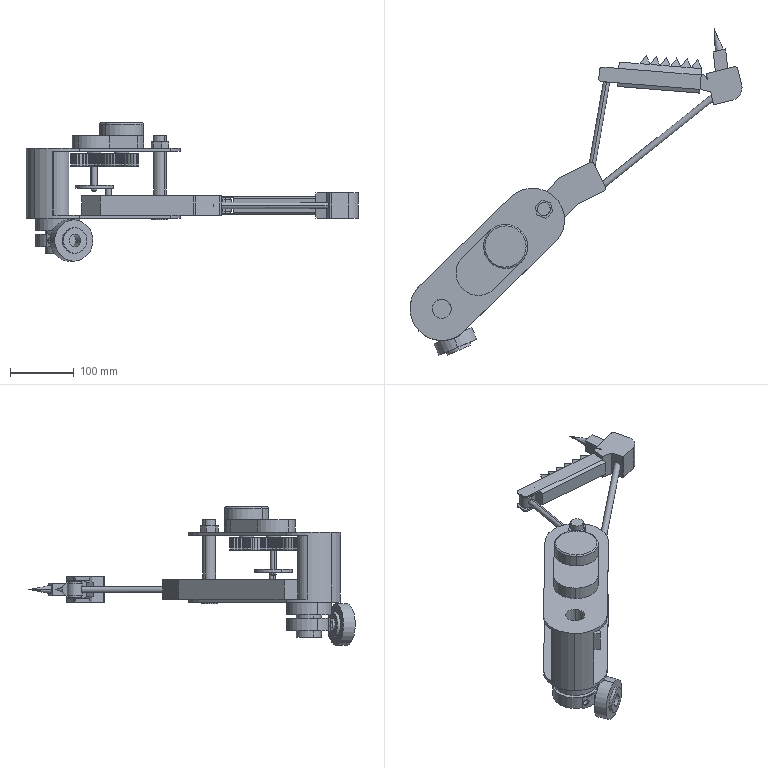Part | SolidWorks | 14 solids | 544 faces | box 522.188 x 513.353 x 217.5 mm | volume 1544826 mm3 | cylinder 378 | plane 158 | torus 6 | cone 2 | commonest cylinder face diameters 20 x97 28 x74 64.998 x35 74 x35 10 x30 44.998 x25